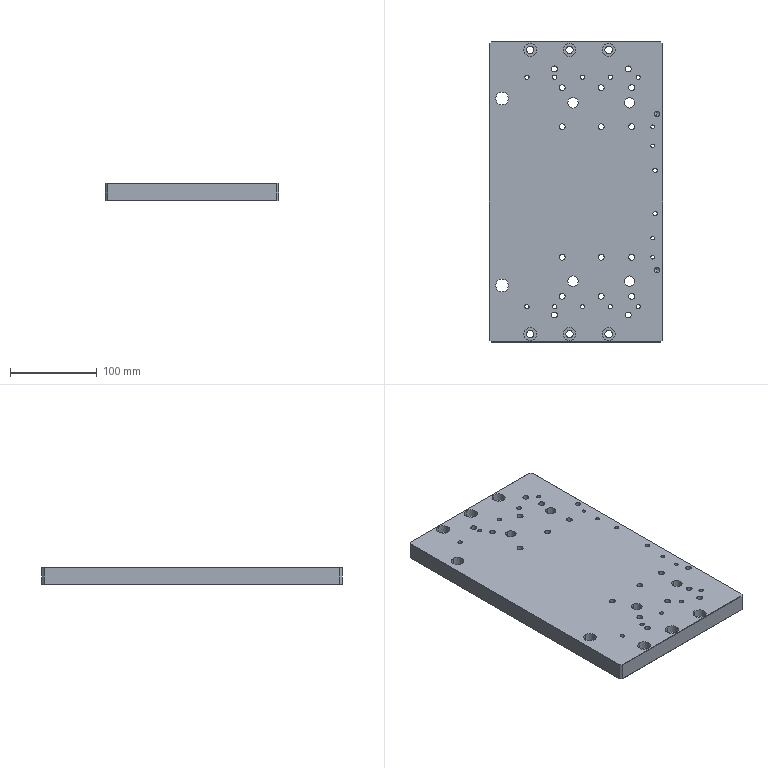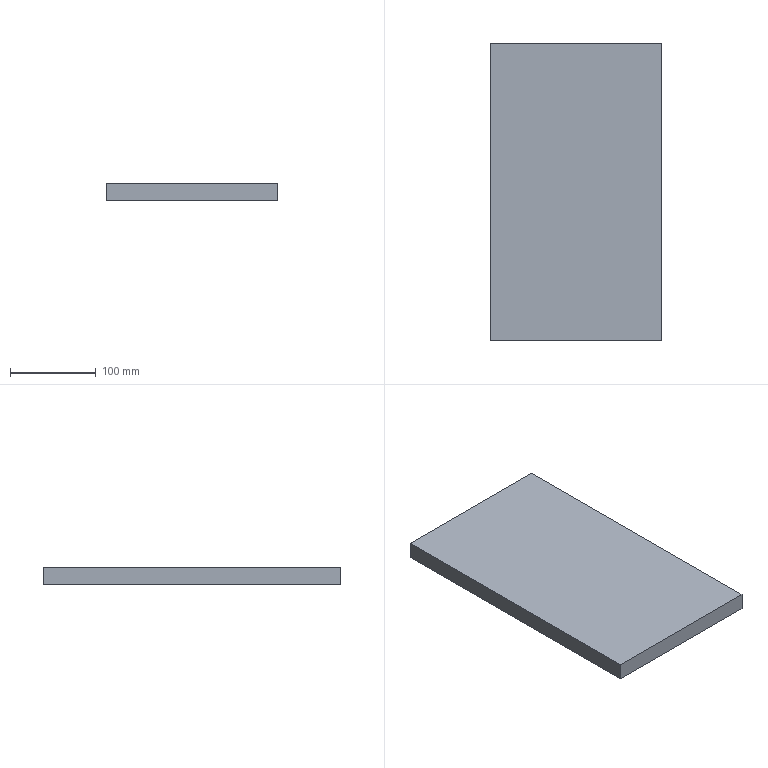CAM job | NX | 3-axis milling, drilling | part box 200 x 346 x 20 mm | stock box 200 x 346 x 20 mm
Tools:
number,name,description,diameter,corner_radius,flute_length,length,flutes
21,ZXZ,Milling Tool-5 Parameters,6.0,0.0,50.0,75.0,2
16,8.4ZT,Drilling Tool,8.4,0.0,35.0,50.0,2
10,6.8ZT,Drilling Tool,6.8,0.0,35.0,50.0,2
5,5.0ZT,Drilling Tool,5.0,0.0,35.0,50.0,2
4,4.2ZT,Drilling Tool,4.2,0.0,35.0,50.0,2
17,12.0ZT,Drilling Tool,12.0,0.0,35.0,50.0,2
13,D8,Milling Tool-5 Parameters,8.0,0.0,50.0,75.0,2
18,14.5ZT,Drilling Tool,14.5,0.0,35.0,50.0,2
11,D4,Milling Tool-5 Parameters,4.0,0.0,50.0,75.0,2
1,D6A45,Milling Tool-5 Parameters,6.0,0.0,50.0,75.0,2
24,D10M14铣牙刀,Thread Mill,10.0,0.0,2.0,50.0,2
9,D10M16铣牙刀,Thread Mill,10.0,0.0,1.5,50.0,2
7,3.5ZT,Drilling Tool,3.5,0.0,35.0,50.0,2
3,D3,Milling Tool-5 Parameters,3.0,0.0,50.0,75.0,2
Operations:
program,operation,operation_type,tool,method,geometry_group,spindle_rpm,surface_speed,feed_per_tooth,feed_cut,feed_plunge,cut_length_mm,path_length_mm,cut_time_min,machine_time_min
1,DRILLING,Operation,ZXZ,METHOD,A,3500.0,65.0,0.0429,300.0,0.0,184.0,1821.762,0.6133,0.7771
1,DRILLING_COPY,Operation,8.4ZT,METHOD,A,1500.0,28.0,0.0667,200.0,0.0,159.142,900.697,0.7957,0.8699
1,DRILLING_COPY_COPY,Operation,6.8ZT,METHOD,A,1500.0,28.0,0.0667,200.0,0.0,416.687,1596.097,2.083,2.201
1,DRILLING_COPY_COPY_COPY,Operation,5.0ZT,METHOD,A,1500.0,28.0,0.0667,200.0,0.0,306.026,1229.871,1.53,1.623
1,DRILLING_COPY_COPY_COPY_COPY,Operation,5.0ZT,METHOD,A,1500.0,28.0,0.0667,200.0,0.0,39.004,321.034,0.195,0.2232
1,DRILLING_COPY_COPY_COPY_COPY_COPY,Operation,4.2ZT,METHOD,A,2122.0,28.0,0.0471,200.0,0.0,103.047,425.544,0.5152,0.5475
1,DRILLING_COPY_COPY_1,Operation,12.0ZT,METHOD,A,1500.0,28.0,0.0667,200.0,0.0,110.421,625.002,0.5521,0.6036
1,DRILLING_COPY_COPY_1_COPY,Operation,14.5ZT,METHOD,A,1500.0,28.0,0.0667,200.0,0.0,56.712,391.446,0.2836,0.317
1,HOLE_MILLING,CylinderMilling,D8,METHOD,A,3500.0,87.0,0.3143,2200.0,100.0,6465.657,7383.657,2.939,3.031
1,HOLE_MILLING_COPY,CylinderMilling,D4,METHOD,A,5000.0,62.0,0.18,1800.0,100.0,1186.048,1515.048,0.6589,0.6918
1,PLANAR_MILL,PlanarMilling,D6A45,METHOD,A,7500.0,141.0,0.0833,1250.0,100.0,1403.086,5252.944,1.123,1.508
1,PLANAR_MILL_COPY,PlanarMilling,D6A45,METHOD,A,7500.0,141.0,0.0833,1250.0,100.0,1099.308,1155.308,0.8794,0.885
1,刀补11,CylinderMilling,D4,METHOD,A,5000.0,62.0,0.18,1800.0,100.0,850.572,1179.572,0.4725,0.5054
1,刀补24,ThreadMilling,D10M14铣牙刀,METHOD,A,2500.0,78.0,0.1,500.0,100.0,1405.465,2230.858,2.811,2.893
1,刀补9,ThreadMilling,D10M16铣牙刀,METHOD,A,2500.0,78.0,0.1,500.0,100.0,1022.206,1437.908,2.044,2.086
2,DRILLING_COPY_1,Operation,ZXZ,METHOD,B,3500.0,65.0,0.0429,300.0,0.0,16.0,251.45,0.0533,0.0769
2,DRILLING_COPY_COPY_COPY_COPY_COPY_COPY,Operation,3.5ZT,METHOD,B,2000.0,21.0,0.0325,130.0,0.0,48.206,315.862,0.3708,0.3976
2,PLANAR_MILL_COPY_1,PlanarMilling,D6A45,METHOD,B,7500.0,141.0,0.0833,1250.0,100.0,1311.886,5279.689,1.05,1.446
2,PLANAR_MILL_COPY_1_COPY,PlanarMilling,D6A45,METHOD,B,7500.0,141.0,0.0833,1250.0,100.0,1099.308,1155.308,0.8794,0.885
2,刀补11_COPY,CylinderMilling,D3,METHOD,B,6578.0,62.0,0.0912,1200.0,100.0,957.101,1377.101,0.7976,0.8396